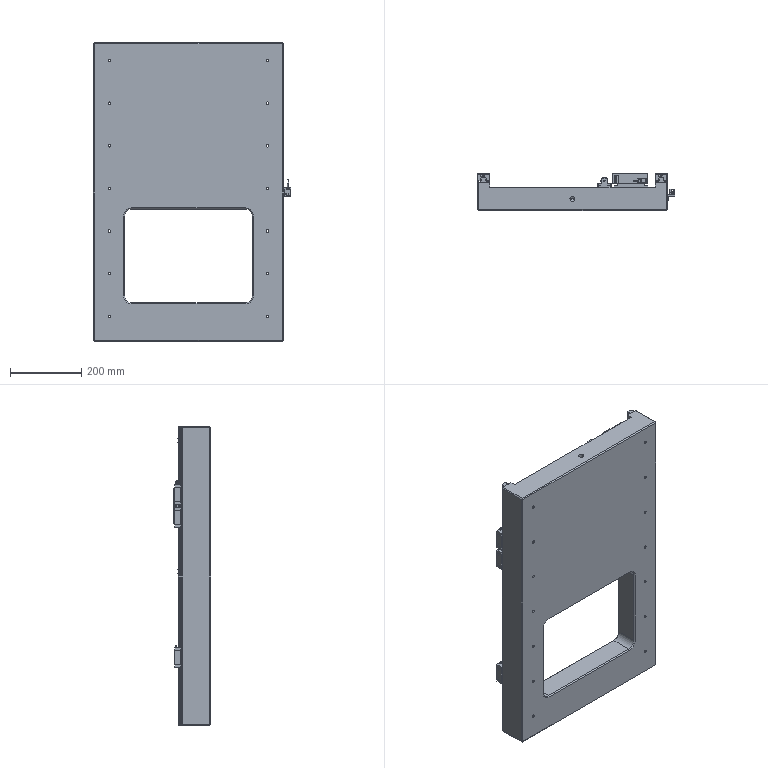Part | NX | features BREP 22 | 28 solids | 1646 faces | box 555 x 105 x 840 mm | volume 24900873 mm3 | plane 917 | cylinder 543 | cone 174 | torus 12 | commonest cylinder face diameters 3.3 x100 4.5 x92 8.1 x56 4.8 x36 7 x28 15 x28